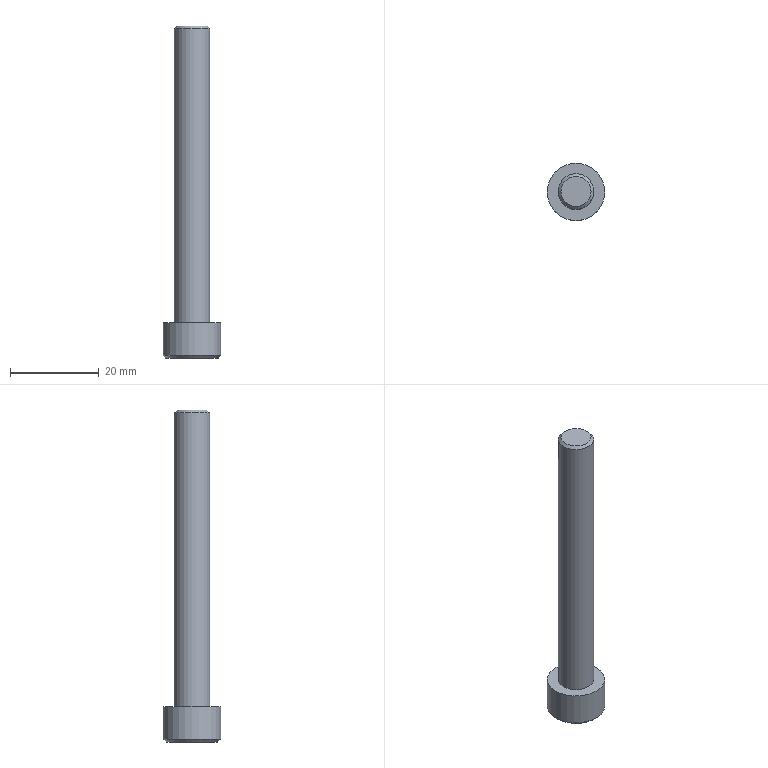Part | STEP file | M8.00-75.00 | 1 solid | 14 faces | box 13 x 13 x 75 mm | volume 4258 mm3 | plane 10 | cylinder 2 | cone 2 | commonest cylinder face diameters 8 x1 13 x1